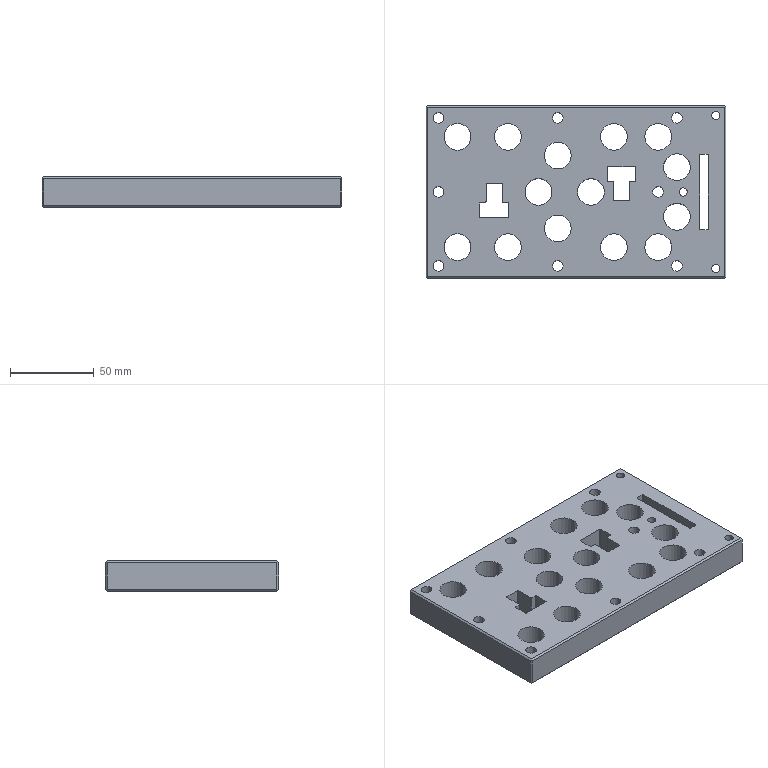Part | Creo | features DATUM PLANE 3, CHAMFER 1, COORDINATE SYSTEM 1, CURVE 1, PROTRUSION 1 | 1 solid | 108 faces | box 179.25 x 103.5 x 18 mm | volume 263298 mm3 | cylinder 70 | plane 38 | commonest cylinder face diameters 16 x28 0.75 x16 6.375 x16 4.875 x6 1.5 x4